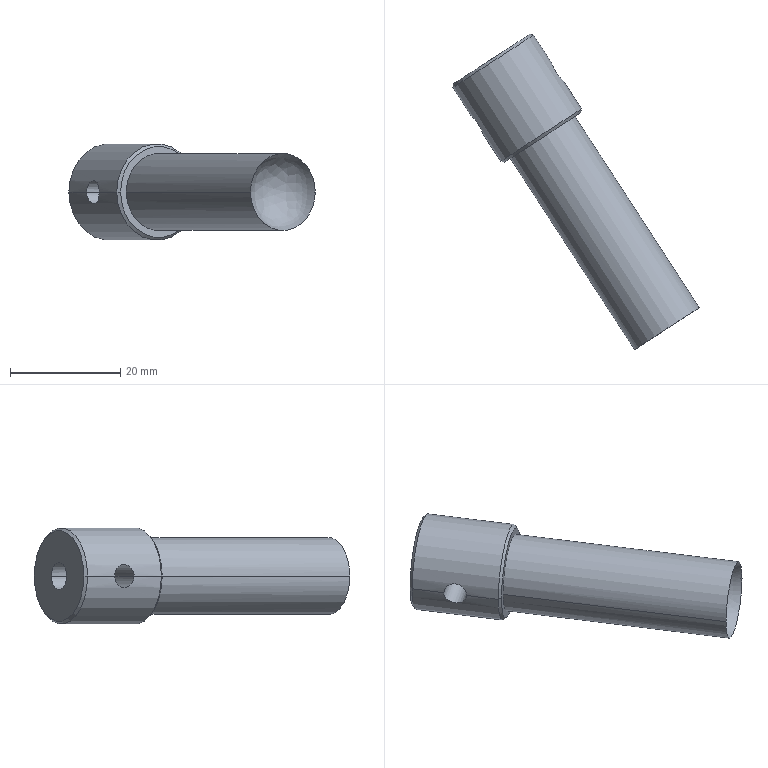Part | STEP file | CPR14030_1-A - longo | 1 solid | 19 faces | volume 9631 mm3 | cylinder 8 | cone 6 | plane 4 | spline 1 | commonest cylinder face diameters 4.2 x2 5 x2 14 x2 17.5 x2